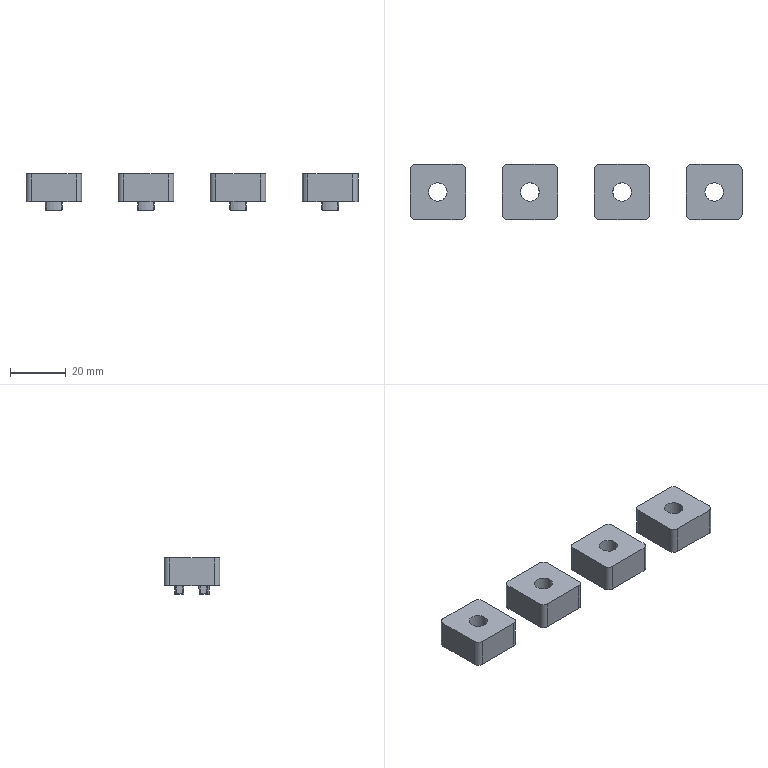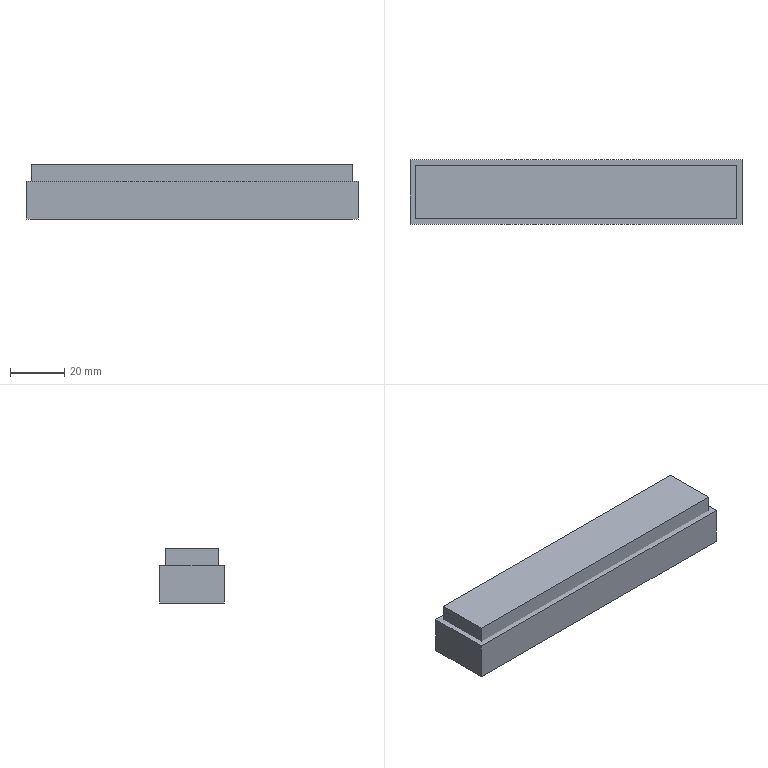CAM job | NX | 3-axis milling, drilling | part box 118.91 x 19.91 x 13 mm | stock box 122.91 x 23.91 x 20 mm
Tools:
number,name,description,diameter,corner_radius,flute_length,length,flutes
19,D80,Milling Tool-5 Parameters,80.0,0.0,50.0,75.0,2
15,D10,Milling Tool-5 Parameters,10.0,0.0,50.0,75.0,2
14,D10JING,Milling Tool-5 Parameters,10.0,0.0,50.0,75.0,2
1,D6A45,Milling Tool-5 Parameters,6.0,0.0,50.0,75.0,2
16,6.6ZT,Drilling Tool,6.6,0.0,35.0,50.0,2
12,D6,Milling Tool-5 Parameters,6.0,0.0,50.0,75.0,2
17,D4R0.5,Milling Tool-5 Parameters,4.0,0.5,50.0,75.0,2
Operations:
program,operation,operation_type,tool,method,geometry_group,spindle_rpm,surface_speed,feed_per_tooth,feed_cut,feed_plunge,cut_length_mm,path_length_mm,cut_time_min,machine_time_min
1,FLOOR_WALL,VolumeBased25DMillingOperation,D80,METHOD,A,6500.0,1633.0,0.1154,1500.0,100.0,214.91,268.91,0.1433,0.1487
1,ZLEVEL_PROFILE,ZLevelMilling,D10,METHOD,A,9500.0,298.0,0.1579,3000.0,1000.0,6262.981,6841.523,2.215,2.273
1,ZLEVEL_PROFILE_1,ZLevelMilling,D10JING,METHOD,A,9500.0,298.0,0.0789,1500.0,1000.0,465.129,925.685,0.3157,0.3617
1,DRILLING,Operation,D6A45,METHOD,A,5000.0,94.0,0.025,250.0,0.0,16.0,200.408,0.064,0.0824
1,DRILLING_COPY,Operation,6.6ZT,METHOD,A,2004.0,41.0,0.0624,250.0,0.0,77.931,324.271,0.3117,0.3364
1,FLOOR_WALL_1,VolumeBased25DMillingOperation,D6,METHOD,A,9500.0,179.0,0.1316,2500.0,1000.0,5803.894,6708.489,2.557,2.647
1,FLOOR_WALL_1_COPY,VolumeBased25DMillingOperation,D6,METHOD,A,9500.0,179.0,0.0789,1500.0,1000.0,1220.876,2771.296,0.8777,1.033
1,ZLEVEL_PROFILE_1_1,ZLevelMilling,D4R0.5,METHOD,A,9500.0,119.0,0.1579,3000.0,100.0,6793.627,7634.104,2.264,2.349
1,PLANAR_MILL_COPY_COPY,PlanarMilling,D6A45,METHOD,A,9500.0,179.0,0.0658,1250.0,100.0,223.691,830.868,0.179,0.2397
1,PLANAR_MILL_COPY_COPY_COPY,PlanarMilling,D6A45,METHOD,A,9500.0,179.0,0.0658,1250.0,100.0,354.598,733.882,0.2837,0.3216
2,FLOOR_WALL_COPY,VolumeBased25DMillingOperation,D80,METHOD,B,6500.0,1633.0,0.1154,1500.0,100.0,1476.37,3041.832,0.9842,1.141
2,PLANAR_MILL_COPY_COPY_COPY_COPY,PlanarMilling,D6A45,METHOD,B,9500.0,179.0,0.0658,1250.0,100.0,428.828,1046.313,0.3431,0.4048